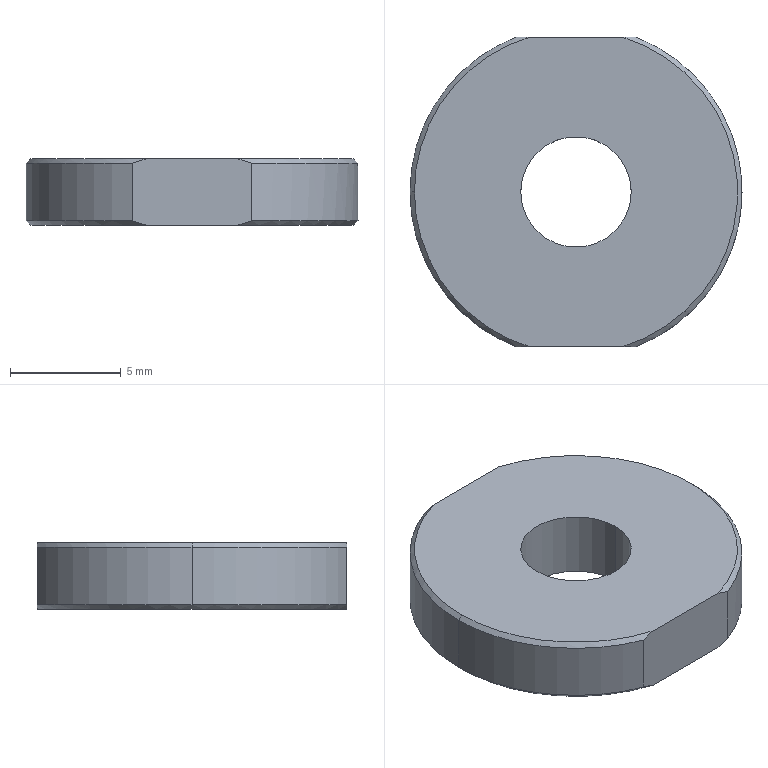Part | STEP file | 11-FG-E04611 | 1 solid | 15 faces | box 15 x 14 x 3 mm | volume 458.934 mm3 | cone 6 | cylinder 5 | plane 4 | commonest cylinder face diameters 15 x3 5 x2
STEP:
#1=CARTESIAN_POINT('',(-7.3,0.,3.));
#2=VERTEX_POINT('',#1);
#3=CARTESIAN_POINT('',(-2.071,-7.,3.));
#4=VERTEX_POINT('',#3);
#5=CARTESIAN_POINT('',(0.,0.,3.));
#6=DIRECTION('',(0.,0.,1.));
#7=DIRECTION('',(1.,0.,0.));
#8=AXIS2_PLACEMENT_3D('',#5,#6,#7);
#9=CIRCLE('',#8,7.3);
#10=EDGE_CURVE('',#2,#4,#9,.T.);
#11=ORIENTED_EDGE('',*,*,#10,.F.);
#12=CARTESIAN_POINT('',(-7.5,0.,2.8));
#13=VERTEX_POINT('',#12);
#14=CARTESIAN_POINT('',(-7.3,0.,3.));
#15=DIRECTION('',(-0.7071,0.,-0.7071));
#16=VECTOR('',#15,1000.);
#17=LINE('',#14,#16);
#18=EDGE_CURVE('',#2,#13,#17,.T.);
#19=ORIENTED_EDGE('',*,*,#18,.T.);
#20=CARTESIAN_POINT('',(-2.693,-7.,2.8));
#21=VERTEX_POINT('',#20);
#22=CARTESIAN_POINT('',(0.,0.,2.8));
#23=DIRECTION('',(0.,0.,-1.));
#24=DIRECTION('',(1.,0.,0.));
#25=AXIS2_PLACEMENT_3D('',#22,#23,#24);
#26=CIRCLE('',#25,7.5);
#27=EDGE_CURVE('',#21,#13,#26,.T.);
#28=ORIENTED_EDGE('',*,*,#27,.F.);
#29=CARTESIAN_POINT('',(-2.071,-7.,3.));
#30=CARTESIAN_POINT('',(-2.28,-7.,2.941));
#31=CARTESIAN_POINT('',(-2.487,-7.,2.874));
#32=CARTESIAN_POINT('',(-2.693,-7.,2.8));
#33=B_SPLINE_CURVE_WITH_KNOTS('',3,(#29,#30,#31,#32),.UNSPECIFIED.,.F.,.F.,(4,4),(0.008463,0.009111),.UNSPECIFIED.);
#34=EDGE_CURVE('',#4,#21,#33,.T.);
#35=ORIENTED_EDGE('',*,*,#34,.F.);
#36=EDGE_LOOP('',(#11,#19,#28,#35));
#37=FACE_OUTER_BOUND('',#36,.T.);
#38=CARTESIAN_POINT('',(0.,0.,3.));
#39=DIRECTION('',(0.,0.,-1.));
#40=DIRECTION('',(-1.,0.,0.));
#41=AXIS2_PLACEMENT_3D('',#38,#39,#40);
#42=CONICAL_SURFACE('',#41,7.3,0.7854);
#43=ADVANCED_FACE('',(#37),#42,.T.);
#44=CARTESIAN_POINT('',(7.3,0.,0.));
#45=VERTEX_POINT('',#44);
#46=CARTESIAN_POINT('',(2.071,-7.,0.));
#47=VERTEX_POINT('',#46);
#48=CARTESIAN_POINT('',(0.,0.,0.));
#49=DIRECTION('',(0.,0.,-1.));
#50=DIRECTION('',(1.,0.,0.));
#51=AXIS2_PLACEMENT_3D('',#48,#49,#50);
#52=CIRCLE('',#51,7.3);
#53=EDGE_CURVE('',#45,#47,#52,.T.);
#54=ORIENTED_EDGE('',*,*,#53,.F.);
#55=CARTESIAN_POINT('',(7.5,0.,0.2));
#56=VERTEX_POINT('',#55);
#57=CARTESIAN_POINT('',(7.5,0.,0.2));
#58=DIRECTION('',(0.7071,0.,0.7071));
#59=VECTOR('',#58,1000.);
#60=LINE('',#57,#59);
#61=EDGE_CURVE('',#45,#56,#60,.T.);
#62=ORIENTED_EDGE('',*,*,#61,.T.);
#63=CARTESIAN_POINT('',(2.693,-7.,0.2));
#64=VERTEX_POINT('',#63);
#65=CARTESIAN_POINT('',(0.,0.,0.2));
#66=DIRECTION('',(0.,0.,1.));
#67=DIRECTION('',(1.,0.,0.));
#68=AXIS2_PLACEMENT_3D('',#65,#66,#67);
#69=CIRCLE('',#68,7.5);
#70=EDGE_CURVE('',#64,#56,#69,.T.);
#71=ORIENTED_EDGE('',*,*,#70,.F.);
#72=CARTESIAN_POINT('',(2.071,-7.,0.));
#73=CARTESIAN_POINT('',(2.28,-7.,0.05922));
#74=CARTESIAN_POINT('',(2.487,-7.,0.1262));
#75=CARTESIAN_POINT('',(2.693,-7.,0.2));
#76=B_SPLINE_CURVE_WITH_KNOTS('',3,(#72,#73,#74,#75),.UNSPECIFIED.,.F.,.F.,(4,4),(0.008463,0.009111),.UNSPECIFIED.);
#77=EDGE_CURVE('',#47,#64,#76,.T.);
#78=ORIENTED_EDGE('',*,*,#77,.F.);
#79=EDGE_LOOP('',(#54,#62,#71,#78));
#80=FACE_OUTER_BOUND('',#79,.T.);
#81=CARTESIAN_POINT('',(0.,0.,0.2));
#82=DIRECTION('',(0.,0.,1.));
#83=DIRECTION('',(1.,0.,0.));
#84=AXIS2_PLACEMENT_3D('',#81,#82,#83);
#85=CONICAL_SURFACE('',#84,7.5,0.7854);
#86=ADVANCED_FACE('',(#80),#85,.T.);
#87=CARTESIAN_POINT('',(-2.5,0.,0.));
#88=VERTEX_POINT('',#87);
#89=CARTESIAN_POINT('',(2.5,0.,0.));
#90=VERTEX_POINT('',#89);
#91=CARTESIAN_POINT('',(0.,0.,0.));
#92=DIRECTION('',(0.,0.,1.));
#93=DIRECTION('',(1.,0.,0.));
#94=AXIS2_PLACEMENT_3D('',#91,#92,#93);
#95=CIRCLE('',#94,2.5);
#96=EDGE_CURVE('',#88,#90,#95,.T.);
#97=ORIENTED_EDGE('',*,*,#96,.F.);
#98=CARTESIAN_POINT('',(-2.5,0.,3.));
#99=VERTEX_POINT('',#98);
#100=CARTESIAN_POINT('',(-2.5,0.,3.));
#101=DIRECTION('',(0.,0.,1.));
#102=VECTOR('',#101,1000.);
#103=LINE('',#100,#102);
#104=EDGE_CURVE('',#88,#99,#103,.T.);
#105=ORIENTED_EDGE('',*,*,#104,.T.);
#106=CARTESIAN_POINT('',(2.5,0.,3.));
#107=VERTEX_POINT('',#106);
#108=CARTESIAN_POINT('',(0.,0.,3.));
#109=DIRECTION('',(0.,0.,1.));
#110=DIRECTION('',(1.,0.,0.));
#111=AXIS2_PLACEMENT_3D('',#108,#109,#110);
#112=CIRCLE('',#111,2.5);
#113=EDGE_CURVE('',#99,#107,#112,.T.);
#114=ORIENTED_EDGE('',*,*,#113,.T.);
#115=CARTESIAN_POINT('',(2.5,0.,3.));
#116=DIRECTION('',(0.,0.,1.));
#117=VECTOR('',#116,1000.);
#118=LINE('',#115,#117);
#119=EDGE_CURVE('',#90,#107,#118,.T.);
#120=ORIENTED_EDGE('',*,*,#119,.F.);
#121=EDGE_LOOP('',(#97,#105,#114,#120));
#122=FACE_OUTER_BOUND('',#121,.T.);
#123=CARTESIAN_POINT('',(0.,0.,3.));
#124=DIRECTION('',(0.,0.,1.));
#125=DIRECTION('',(1.,0.,0.));
#126=AXIS2_PLACEMENT_3D('',#123,#124,#125);
#127=CYLINDRICAL_SURFACE('',#126,2.5);
#128=ADVANCED_FACE('',(#122),#127,.F.);
#129=ORIENTED_EDGE('',*,*,#27,.T.);
#130=CARTESIAN_POINT('',(-7.5,0.,0.2));
#131=VERTEX_POINT('',#130);
#132=CARTESIAN_POINT('',(-7.5,0.,3.));
#133=DIRECTION('',(0.,0.,-1.));
#134=VECTOR('',#133,1000.);
#135=LINE('',#132,#134);
#136=EDGE_CURVE('',#13,#131,#135,.T.);
#137=ORIENTED_EDGE('',*,*,#136,.T.);
#138=CARTESIAN_POINT('',(-2.693,-7.,0.2));
#139=VERTEX_POINT('',#138);
#140=CARTESIAN_POINT('',(0.,0.,0.2));
#141=DIRECTION('',(0.,0.,1.));
#142=DIRECTION('',(1.,0.,0.));
#143=AXIS2_PLACEMENT_3D('',#140,#141,#142);
#144=CIRCLE('',#143,7.5);
#145=EDGE_CURVE('',#131,#139,#144,.T.);
#146=ORIENTED_EDGE('',*,*,#145,.T.);
#147=CARTESIAN_POINT('',(-2.693,-7.,-1.));
#148=DIRECTION('',(0.,0.,1.));
#149=VECTOR('',#148,1000.);
#150=LINE('',#147,#149);
#151=EDGE_CURVE('',#139,#21,#150,.T.);
#152=ORIENTED_EDGE('',*,*,#151,.T.);
#153=EDGE_LOOP('',(#129,#137,#146,#152));
#154=FACE_OUTER_BOUND('',#153,.T.);
#155=CARTESIAN_POINT('',(0.,0.,3.));
#156=DIRECTION('',(0.,0.,-1.));
#157=DIRECTION('',(-1.,0.,0.));
#158=AXIS2_PLACEMENT_3D('',#155,#156,#157);
#159=CYLINDRICAL_SURFACE('',#158,7.5);
#160=ADVANCED_FACE('',(#154),#159,.T.);
#161=CARTESIAN_POINT('',(2.693,7.,2.8));
#162=VERTEX_POINT('',#161);
#163=CARTESIAN_POINT('',(2.693,-7.,2.8));
#164=VERTEX_POINT('',#163);
#165=CARTESIAN_POINT('',(0.,0.,2.8));
#166=DIRECTION('',(0.,0.,-1.));
#167=DIRECTION('',(1.,0.,0.));
#168=AXIS2_PLACEMENT_3D('',#165,#166,#167);
#169=CIRCLE('',#168,7.5);
#170=EDGE_CURVE('',#162,#164,#169,.T.);
#171=ORIENTED_EDGE('',*,*,#170,.T.);
#172=CARTESIAN_POINT('',(2.693,-7.,-1.));
#173=DIRECTION('',(0.,0.,1.));
#174=VECTOR('',#173,1000.);
#175=LINE('',#172,#174);
#176=EDGE_CURVE('',#64,#164,#175,.T.);
#177=ORIENTED_EDGE('',*,*,#176,.F.);
#178=ORIENTED_EDGE('',*,*,#70,.T.);
#179=CARTESIAN_POINT('',(2.693,7.,0.2));
#180=VERTEX_POINT('',#179);
#181=CARTESIAN_POINT('',(0.,0.,0.2));
#182=DIRECTION('',(0.,0.,1.));
#183=DIRECTION('',(1.,0.,0.));
#184=AXIS2_PLACEMENT_3D('',#181,#182,#183);
#185=CIRCLE('',#184,7.5);
#186=EDGE_CURVE('',#56,#180,#185,.T.);
#187=ORIENTED_EDGE('',*,*,#186,.T.);
#188=CARTESIAN_POINT('',(2.693,7.,-1.));
#189=DIRECTION('',(0.,0.,1.));
#190=VECTOR('',#189,1000.);
#191=LINE('',#188,#190);
#192=EDGE_CURVE('',#180,#162,#191,.T.);
#193=ORIENTED_EDGE('',*,*,#192,.T.);
#194=EDGE_LOOP('',(#171,#177,#178,#187,#193));
#195=FACE_OUTER_BOUND('',#194,.T.);
#196=CARTESIAN_POINT('',(0.,0.,3.));
#197=DIRECTION('',(0.,0.,-1.));
#198=DIRECTION('',(-1.,0.,0.));
#199=AXIS2_PLACEMENT_3D('',#196,#197,#198);
#200=CYLINDRICAL_SURFACE('',#199,7.5);
#201=ADVANCED_FACE('',(#195),#200,.T.);
#202=CARTESIAN_POINT('',(-2.071,-7.,0.));
#203=VERTEX_POINT('',#202);
#204=CARTESIAN_POINT('',(-2.693,-7.,0.2));
#205=CARTESIAN_POINT('',(-2.489,-7.,0.1268));
#206=CARTESIAN_POINT('',(-2.281,-7.,0.05945));
#207=CARTESIAN_POINT('',(-2.071,-7.,0.));
#208=B_SPLINE_CURVE_WITH_KNOTS('',3,(#204,#205,#206,#207),.UNSPECIFIED.,.F.,.F.,(4,4),(0.003639,0.004286),.UNSPECIFIED.);
#209=EDGE_CURVE('',#139,#203,#208,.T.);
#210=ORIENTED_EDGE('',*,*,#209,.F.);
#211=ORIENTED_EDGE('',*,*,#145,.F.);
#212=CARTESIAN_POINT('',(-2.693,7.,0.2));
#213=VERTEX_POINT('',#212);
#214=CARTESIAN_POINT('',(0.,0.,0.2));
#215=DIRECTION('',(0.,0.,1.));
#216=DIRECTION('',(1.,0.,0.));
#217=AXIS2_PLACEMENT_3D('',#214,#215,#216);
#218=CIRCLE('',#217,7.5);
#219=EDGE_CURVE('',#213,#131,#218,.T.);
#220=ORIENTED_EDGE('',*,*,#219,.F.);
#221=CARTESIAN_POINT('',(-2.071,7.,0.));
#222=VERTEX_POINT('',#221);
#223=CARTESIAN_POINT('',(-2.071,7.,0.));
#224=CARTESIAN_POINT('',(-2.28,7.,0.05922));
#225=CARTESIAN_POINT('',(-2.487,7.,0.1262));
#226=CARTESIAN_POINT('',(-2.693,7.,0.2));
#227=B_SPLINE_CURVE_WITH_KNOTS('',3,(#223,#224,#225,#226),.UNSPECIFIED.,.F.,.F.,(4,4),(0.008463,0.009111),.UNSPECIFIED.);
#228=EDGE_CURVE('',#222,#213,#227,.T.);
#229=ORIENTED_EDGE('',*,*,#228,.F.);
#230=CARTESIAN_POINT('',(0.,0.,0.));
#231=DIRECTION('',(0.,0.,-1.));
#232=DIRECTION('',(1.,0.,0.));
#233=AXIS2_PLACEMENT_3D('',#230,#231,#232);
#234=CIRCLE('',#233,7.3);
#235=EDGE_CURVE('',#203,#222,#234,.T.);
#236=ORIENTED_EDGE('',*,*,#235,.F.);
#237=EDGE_LOOP('',(#210,#211,#220,#229,#236));
#238=FACE_OUTER_BOUND('',#237,.T.);
#239=CARTESIAN_POINT('',(0.,0.,0.2));
#240=DIRECTION('',(0.,0.,1.));
#241=DIRECTION('',(1.,0.,0.));
#242=AXIS2_PLACEMENT_3D('',#239,#240,#241);
#243=CONICAL_SURFACE('',#242,7.5,0.7854);
#244=ADVANCED_FACE('',(#238),#243,.T.);
#245=CARTESIAN_POINT('',(2.071,-7.,3.));
#246=VERTEX_POINT('',#245);
#247=CARTESIAN_POINT('',(2.693,-7.,2.8));
#248=CARTESIAN_POINT('',(2.489,-7.,2.873));
#249=CARTESIAN_POINT('',(2.281,-7.,2.941));
#250=CARTESIAN_POINT('',(2.071,-7.,3.));
#251=B_SPLINE_CURVE_WITH_KNOTS('',3,(#247,#248,#249,#250),.UNSPECIFIED.,.F.,.F.,(4,4),(0.003639,0.004286),.UNSPECIFIED.);
#252=EDGE_CURVE('',#164,#246,#251,.T.);
#253=ORIENTED_EDGE('',*,*,#252,.F.);
#254=ORIENTED_EDGE('',*,*,#170,.F.);
#255=CARTESIAN_POINT('',(2.071,7.,3.));
#256=VERTEX_POINT('',#255);
#257=CARTESIAN_POINT('',(2.071,7.,3.));
#258=CARTESIAN_POINT('',(2.28,7.,2.941));
#259=CARTESIAN_POINT('',(2.487,7.,2.874));
#260=CARTESIAN_POINT('',(2.693,7.,2.8));
#261=B_SPLINE_CURVE_WITH_KNOTS('',3,(#257,#258,#259,#260),.UNSPECIFIED.,.F.,.F.,(4,4),(0.008463,0.009111),.UNSPECIFIED.);
#262=EDGE_CURVE('',#256,#162,#261,.T.);
#263=ORIENTED_EDGE('',*,*,#262,.F.);
#264=CARTESIAN_POINT('',(0.,0.,3.));
#265=DIRECTION('',(0.,0.,1.));
#266=DIRECTION('',(1.,0.,0.));
#267=AXIS2_PLACEMENT_3D('',#264,#265,#266);
#268=CIRCLE('',#267,7.3);
#269=EDGE_CURVE('',#246,#256,#268,.T.);
#270=ORIENTED_EDGE('',*,*,#269,.F.);
#271=EDGE_LOOP('',(#253,#254,#263,#270));
#272=FACE_OUTER_BOUND('',#271,.T.);
#273=CARTESIAN_POINT('',(0.,0.,3.));
#274=DIRECTION('',(0.,0.,-1.));
#275=DIRECTION('',(-1.,0.,0.));
#276=AXIS2_PLACEMENT_3D('',#273,#274,#275);
#277=CONICAL_SURFACE('',#276,7.3,0.7854);
#278=ADVANCED_FACE('',(#272),#277,.T.);
#279=ORIENTED_EDGE('',*,*,#136,.F.);
#280=CARTESIAN_POINT('',(-2.693,7.,2.8));
#281=VERTEX_POINT('',#280);
#282=CARTESIAN_POINT('',(0.,0.,2.8));
#283=DIRECTION('',(0.,0.,-1.));
#284=DIRECTION('',(1.,0.,0.));
#285=AXIS2_PLACEMENT_3D('',#282,#283,#284);
#286=CIRCLE('',#285,7.5);
#287=EDGE_CURVE('',#13,#281,#286,.T.);
#288=ORIENTED_EDGE('',*,*,#287,.T.);
#289=CARTESIAN_POINT('',(-2.693,7.,-1.));
#290=DIRECTION('',(0.,0.,1.));
#291=VECTOR('',#290,1000.);
#292=LINE('',#289,#291);
#293=EDGE_CURVE('',#213,#281,#292,.T.);
#294=ORIENTED_EDGE('',*,*,#293,.F.);
#295=ORIENTED_EDGE('',*,*,#219,.T.);
#296=EDGE_LOOP('',(#279,#288,#294,#295));
#297=FACE_OUTER_BOUND('',#296,.T.);
#298=CARTESIAN_POINT('',(0.,0.,3.));
#299=DIRECTION('',(0.,0.,-1.));
#300=DIRECTION('',(-1.,0.,0.));
#301=AXIS2_PLACEMENT_3D('',#298,#299,#300);
#302=CYLINDRICAL_SURFACE('',#301,7.5);
#303=ADVANCED_FACE('',(#297),#302,.T.);
#304=CARTESIAN_POINT('',(-2.693,-7.,3.));
#305=DIRECTION('',(-1.,0.,0.));
#306=VECTOR('',#305,1000.);
#307=LINE('',#304,#306);
#308=EDGE_CURVE('',#246,#4,#307,.T.);
#309=ORIENTED_EDGE('',*,*,#308,.F.);
#310=ORIENTED_EDGE('',*,*,#269,.T.);
#311=CARTESIAN_POINT('',(-2.071,7.,3.));
#312=VERTEX_POINT('',#311);
#313=CARTESIAN_POINT('',(-2.693,7.,3.));
#314=DIRECTION('',(1.,0.,0.));
#315=VECTOR('',#314,1000.);
#316=LINE('',#313,#315);
#317=EDGE_CURVE('',#312,#256,#316,.T.);
#318=ORIENTED_EDGE('',*,*,#317,.F.);
#319=CARTESIAN_POINT('',(0.,0.,3.));
#320=DIRECTION('',(0.,0.,1.));
#321=DIRECTION('',(1.,0.,0.));
#322=AXIS2_PLACEMENT_3D('',#319,#320,#321);
#323=CIRCLE('',#322,7.3);
#324=EDGE_CURVE('',#312,#2,#323,.T.);
#325=ORIENTED_EDGE('',*,*,#324,.T.);
#326=ORIENTED_EDGE('',*,*,#10,.T.);
#327=EDGE_LOOP('',(#309,#310,#318,#325,#326));
#328=FACE_OUTER_BOUND('',#327,.T.);
#329=CARTESIAN_POINT('',(0.,0.,3.));
#330=DIRECTION('',(0.,0.,1.));
#331=DIRECTION('',(1.,0.,0.));
#332=AXIS2_PLACEMENT_3D('',#329,#330,#331);
#333=CIRCLE('',#332,2.5);
#334=EDGE_CURVE('',#107,#99,#333,.T.);
#335=ORIENTED_EDGE('',*,*,#334,.F.);
#336=ORIENTED_EDGE('',*,*,#113,.F.);
#337=EDGE_LOOP('',(#335,#336));
#338=FACE_BOUND('',#337,.T.);
#339=CARTESIAN_POINT('',(0.,0.,3.));
#340=DIRECTION('',(0.,0.,1.));
#341=DIRECTION('',(1.,0.,0.));
#342=AXIS2_PLACEMENT_3D('',#339,#340,#341);
#343=PLANE('',#342);
#344=ADVANCED_FACE('',(#328,#338),#343,.T.);
#345=CARTESIAN_POINT('',(2.071,7.,0.));
#346=VERTEX_POINT('',#345);
#347=CARTESIAN_POINT('',(0.,0.,0.));
#348=DIRECTION('',(0.,0.,-1.));
#349=DIRECTION('',(1.,0.,0.));
#350=AXIS2_PLACEMENT_3D('',#347,#348,#349);
#351=CIRCLE('',#350,7.3);
#352=EDGE_CURVE('',#346,#45,#351,.T.);
#353=ORIENTED_EDGE('',*,*,#352,.T.);
#354=ORIENTED_EDGE('',*,*,#53,.T.);
#355=CARTESIAN_POINT('',(0.,-7.,0.));
#356=DIRECTION('',(-1.,0.,0.));
#357=VECTOR('',#356,1000.);
#358=LINE('',#355,#357);
#359=EDGE_CURVE('',#47,#203,#358,.T.);
#360=ORIENTED_EDGE('',*,*,#359,.T.);
#361=ORIENTED_EDGE('',*,*,#235,.T.);
#362=CARTESIAN_POINT('',(0.,7.,0.));
#363=DIRECTION('',(1.,0.,0.));
#364=VECTOR('',#363,1000.);
#365=LINE('',#362,#364);
#366=EDGE_CURVE('',#222,#346,#365,.T.);
#367=ORIENTED_EDGE('',*,*,#366,.T.);
#368=EDGE_LOOP('',(#353,#354,#360,#361,#367));
#369=FACE_OUTER_BOUND('',#368,.T.);
#370=CARTESIAN_POINT('',(0.,0.,0.));
#371=DIRECTION('',(0.,0.,1.));
#372=DIRECTION('',(1.,0.,0.));
#373=AXIS2_PLACEMENT_3D('',#370,#371,#372);
#374=CIRCLE('',#373,2.5);
#375=EDGE_CURVE('',#90,#88,#374,.T.);
#376=ORIENTED_EDGE('',*,*,#375,.T.);
#377=ORIENTED_EDGE('',*,*,#96,.T.);
#378=EDGE_LOOP('',(#376,#377));
#379=FACE_BOUND('',#378,.T.);
#380=CARTESIAN_POINT('',(0.,0.,0.));
#381=DIRECTION('',(0.,0.,1.));
#382=DIRECTION('',(1.,0.,0.));
#383=AXIS2_PLACEMENT_3D('',#380,#381,#382);
#384=PLANE('',#383);
#385=ADVANCED_FACE('',(#369,#379),#384,.F.);
#386=ORIENTED_EDGE('',*,*,#104,.F.);
#387=ORIENTED_EDGE('',*,*,#375,.F.);
#388=ORIENTED_EDGE('',*,*,#119,.T.);
#389=ORIENTED_EDGE('',*,*,#334,.T.);
#390=EDGE_LOOP('',(#386,#387,#388,#389));
#391=FACE_OUTER_BOUND('',#390,.T.);
#392=CARTESIAN_POINT('',(0.,0.,3.));
#393=DIRECTION('',(0.,0.,1.));
#394=DIRECTION('',(1.,0.,0.));
#395=AXIS2_PLACEMENT_3D('',#392,#393,#394);
#396=CYLINDRICAL_SURFACE('',#395,2.5);
#397=ADVANCED_FACE('',(#391),#396,.F.);
#398=ORIENTED_EDGE('',*,*,#61,.F.);
#399=ORIENTED_EDGE('',*,*,#352,.F.);
#400=CARTESIAN_POINT('',(2.693,7.,0.2));
#401=CARTESIAN_POINT('',(2.489,7.,0.1268));
#402=CARTESIAN_POINT('',(2.281,7.,0.05945));
#403=CARTESIAN_POINT('',(2.071,7.,0.));
#404=B_SPLINE_CURVE_WITH_KNOTS('',3,(#400,#401,#402,#403),.UNSPECIFIED.,.F.,.F.,(4,4),(0.003639,0.004286),.UNSPECIFIED.);
#405=EDGE_CURVE('',#180,#346,#404,.T.);
#406=ORIENTED_EDGE('',*,*,#405,.F.);
#407=ORIENTED_EDGE('',*,*,#186,.F.);
#408=EDGE_LOOP('',(#398,#399,#406,#407));
#409=FACE_OUTER_BOUND('',#408,.T.);
#410=CARTESIAN_POINT('',(0.,0.,0.2));
#411=DIRECTION('',(0.,0.,1.));
#412=DIRECTION('',(1.,0.,0.));
#413=AXIS2_PLACEMENT_3D('',#410,#411,#412);
#414=CONICAL_SURFACE('',#413,7.5,0.7854);
#415=ADVANCED_FACE('',(#409),#414,.T.);
#416=ORIENTED_EDGE('',*,*,#18,.F.);
#417=ORIENTED_EDGE('',*,*,#324,.F.);
#418=CARTESIAN_POINT('',(-2.693,7.,2.8));
#419=CARTESIAN_POINT('',(-2.489,7.,2.873));
#420=CARTESIAN_POINT('',(-2.281,7.,2.941));
#421=CARTESIAN_POINT('',(-2.071,7.,3.));
#422=B_SPLINE_CURVE_WITH_KNOTS('',3,(#418,#419,#420,#421),.UNSPECIFIED.,.F.,.F.,(4,4),(0.003639,0.004286),.UNSPECIFIED.);
#423=EDGE_CURVE('',#281,#312,#422,.T.);
#424=ORIENTED_EDGE('',*,*,#423,.F.);
#425=ORIENTED_EDGE('',*,*,#287,.F.);
#426=EDGE_LOOP('',(#416,#417,#424,#425));
#427=FACE_OUTER_BOUND('',#426,.T.);
#428=CARTESIAN_POINT('',(0.,0.,3.));
#429=DIRECTION('',(0.,0.,-1.));
#430=DIRECTION('',(-1.,0.,0.));
#431=AXIS2_PLACEMENT_3D('',#428,#429,#430);
#432=CONICAL_SURFACE('',#431,7.3,0.7854);
#433=ADVANCED_FACE('',(#427),#432,.T.);
#434=ORIENTED_EDGE('',*,*,#405,.T.);
#435=ORIENTED_EDGE('',*,*,#366,.F.);
#436=ORIENTED_EDGE('',*,*,#228,.T.);
#437=ORIENTED_EDGE('',*,*,#293,.T.);
#438=ORIENTED_EDGE('',*,*,#423,.T.);
#439=ORIENTED_EDGE('',*,*,#317,.T.);
#440=ORIENTED_EDGE('',*,*,#262,.T.);
#441=ORIENTED_EDGE('',*,*,#192,.F.);
#442=EDGE_LOOP('',(#434,#435,#436,#437,#438,#439,#440,#441));
#443=FACE_OUTER_BOUND('',#442,.T.);
#444=CARTESIAN_POINT('',(-2.693,7.,-1.));
#445=DIRECTION('',(0.,-1.,0.));
#446=DIRECTION('',(0.,0.,-1.));
#447=AXIS2_PLACEMENT_3D('',#444,#445,#446);
#448=PLANE('',#447);
#449=ADVANCED_FACE('',(#443),#448,.F.);
#450=ORIENTED_EDGE('',*,*,#209,.T.);
#451=ORIENTED_EDGE('',*,*,#359,.F.);
#452=ORIENTED_EDGE('',*,*,#77,.T.);
#453=ORIENTED_EDGE('',*,*,#176,.T.);
#454=ORIENTED_EDGE('',*,*,#252,.T.);
#455=ORIENTED_EDGE('',*,*,#308,.T.);
#456=ORIENTED_EDGE('',*,*,#34,.T.);
#457=ORIENTED_EDGE('',*,*,#151,.F.);
#458=EDGE_LOOP('',(#450,#451,#452,#453,#454,#455,#456,#457));
#459=FACE_OUTER_BOUND('',#458,.T.);
#460=CARTESIAN_POINT('',(-2.693,-7.,-1.));
#461=DIRECTION('',(0.,1.,0.));
#462=DIRECTION('',(0.,0.,1.));
#463=AXIS2_PLACEMENT_3D('',#460,#461,#462);
#464=PLANE('',#463);
#465=ADVANCED_FACE('',(#459),#464,.F.);
#466=CLOSED_SHELL('',(#43,#86,#128,#160,#201,#244,#278,#303,#344,#385,#397,#415,#433,#449,#465));
#467=MANIFOLD_SOLID_BREP('',#466);
#468=CARTESIAN_POINT('',(0.,0.,0.));
#469=DIRECTION('',(0.,0.,1.));
#470=DIRECTION('',(1.,0.,0.));
#471=AXIS2_PLACEMENT_3D('',#468,#469,#470);
#472=(LENGTH_UNIT()NAMED_UNIT(*)SI_UNIT(.MILLI.,.METRE.));
#473=UNCERTAINTY_MEASURE_WITH_UNIT(LENGTH_MEASURE(0.00001),#472,'','');
#474=(NAMED_UNIT(*)PLANE_ANGLE_UNIT()SI_UNIT($,.RADIAN.));
#475=(NAMED_UNIT(*)SI_UNIT($,.STERADIAN.)SOLID_ANGLE_UNIT());
#476=(GEOMETRIC_REPRESENTATION_CONTEXT(3)GLOBAL_UNCERTAINTY_ASSIGNED_CONTEXT((#473))GLOBAL_UNIT_ASSIGNED_CONTEXT((#472,#474,#475))REPRESENTATION_CONTEXT('',''));
#477=ADVANCED_BREP_SHAPE_REPRESENTATION('',(#467,#471),#476);